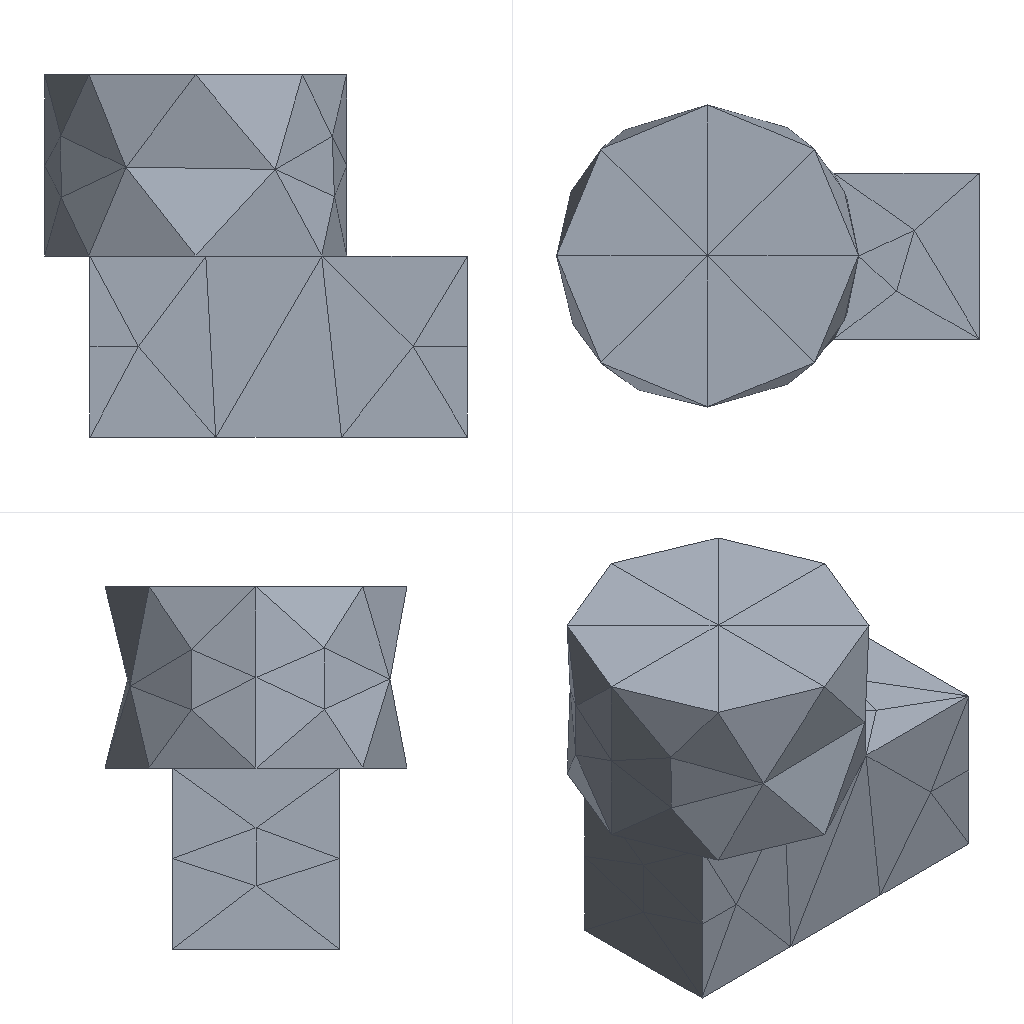Simulation study | ansys mapdl
Set-up summary:
category,name,step,type,value,unit,region
solver,ansys_mapdl
units,mm-N-s-tonne (MPa),,inferred,E=210000 density=
analysis,model,,static
mesh,nodes,,,326
mesh,elements,,,141
element_type,SOLID187,,,141
material,mat 1,,E,210000
material,mat 1,,nu,0.3
load,,model,body load temp,,,all
load,,model,force,"1000 [dir=(0, 0, -1) n=59]",,node list
bc,,model,fixed,"[dofs=UX,UY,UZ n=271]",,node list
Ansys APDL input file, long lists of numbers shortened:
/COM,ANSYS RELEASE 2026 R1           BUILD 26.1      UP20260202       09:08:10
/PREP7
/NOPR
/TITLE,2
ANTYPE, 0
*IF,_CDRDOFF,EQ,1,THEN     !if solid model was read in
_CDRDOFF=             !reset flag, numoffs already performed
*ELSE              !offset database for the following FE model
NUMOFF,NODE,      326
NUMOFF,ELEM,      141
NUMOFF,MAT ,        1
NUMOFF,TYPE,        1
*ENDIF
*SET,_RETURN ,  0.
*SET,_STATUS ,  0.
*SET,_UIQR   ,  59.
*SET,__FLOATPARAMETER__,  326.
DOF,DELETE
ETBLOCK,        1,        1
(2i9,19a9)
        1      187        0        0        0        0        0        0        0        0        0        0        0        0        0        0        0        0        0        0        0
       -1
NBLOCK,6,SOLID,       326,       326
(3i9,6e21.13e3)
        1        0        0 3.6000000000000E+001 0.0000000000000E+000 6.0000000000000E+001
! (325 more lines like these left out)
N,UNBL,LOC,       -1,
EBLOCK,19,SOLID,       141,       141
(19i10)
         1         1         1         1         0         0         0         0        10         0         1       156        68       152       194       241       242       155       173
! (281 more lines like these left out)
        -1
MPTEMP,UNBL, 1, 1,  0.    ,
MPDATA,UNBL, 1,EX  ,       1, 1,  210000.000    ,
MPTEMP,UNBL, 1, 1,  0.    ,
MPDATA,UNBL, 1,NUXY,       1, 1, 0.3    ,
MPTEMP,UNBL, 1, 1,  0.    ,
MPDATA,UNBL, 1,PRXY,       1, 1, 0.3    ,
EXTOPT,ATTR,      0,      0,      0
EXTOPT,ESIZE,  0,  0.
EXTOPT,ACLEAR,      0
TREF,  0.
IRLF,  0
BFUNIF,TEMP,_TINY
ACEL,  0.    ,  0.    ,  0.
OMEGA,  0.    ,  0.    ,  0.
DOMEGA,  0.    ,  0.    ,  0.
CGLOC,  0.    ,  0.    ,  0.
CGOMEGA,  0.    ,  0.    ,  0.
DCGOMG,  0.    ,  0.    ,  0.
KUSE,     0
TIME,  0.
ALPHAD,  0.
BETAD,  0.
DMPRAT,  0.
DMPSTR,  0.
CRPLIM, 0.1    ,   0
CRPLIM,  0.    ,   1
NCNV,     0, 1.000000000E+12,     0,  0.    ,  0.
NEQIT,     0
ERESX,DEFA
DBLOCK,       271
(i9,a6,2(pg16.9))
       21  UX    0.00000000      0.00000000
! (270 more lines like these left out)
       -1
FBLOCK,        59
(i9,a6,2(pg16.9))
      127  FZ   -16.9491525      0.00000000
! (58 more lines like these left out)
       -1
/GO
FINISH
Results summary:
result,analysis_type_db,,,static,unstated
result,n_sets,,,1,unstated
result,load_steps[0].set,load_step=1,,1,unstated
result,load_steps[0].substep,load_step=1,,1,unstated
result,load_steps[0].time,load_step=1,,1,unstated
result,load_steps[0].freq,load_step=1,,1,unstated
result,load_steps[0].max_usum,load_step=1,,0.000514,unstated
result,load_steps[0].max_seqv,load_step=1,,6.19,unstated
result,load_steps[0].reaction_sum.FX,load_step=1,,6.00053e-12,unstated
result,load_steps[0].reaction_sum.FY,load_step=1,,3.43121e-11,unstated
result,load_steps[0].reaction_sum.FZ,load_step=1,,1000,unstated
result,load_steps[0].reaction_sum.MX,load_step=1,,0,unstated
result,load_steps[0].reaction_sum.MY,load_step=1,,0,unstated
result,load_steps[0].reaction_sum.MZ,load_step=1,,0,unstated
result,convergence,,,results present for all listed sets,unstated